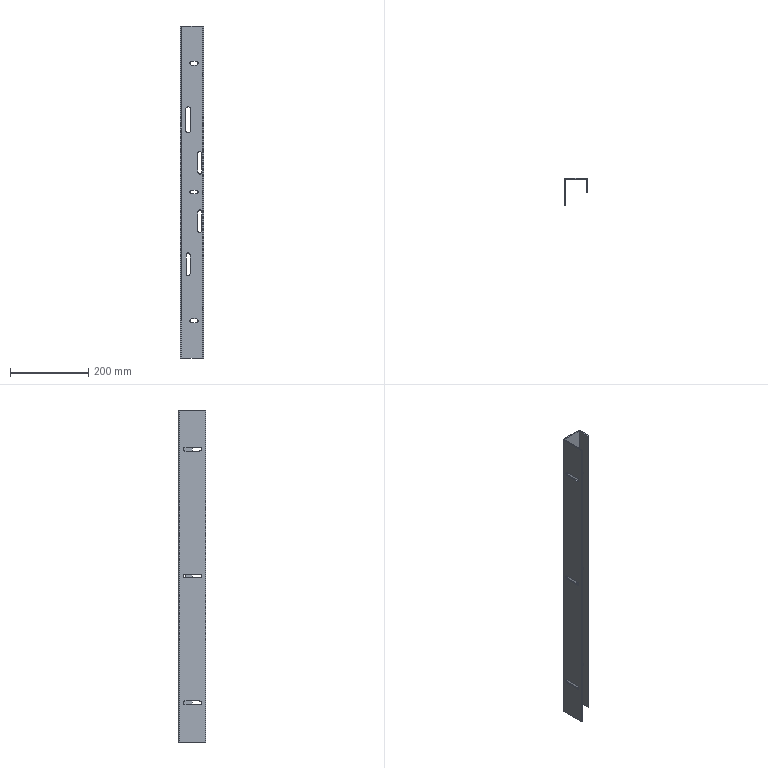Part | SolidWorks | features ICE 3, FlatPattern 1, SMBaseFlange 1, SheetMetal 1 | 1 solid | 71 faces | box 60 x 70 x 850 mm | volume 387976 mm3 | plane 38 | cylinder 33 | commonest cylinder face diameters 10 x21 7 x6 0.4 x2 6.4 x2 14 x2